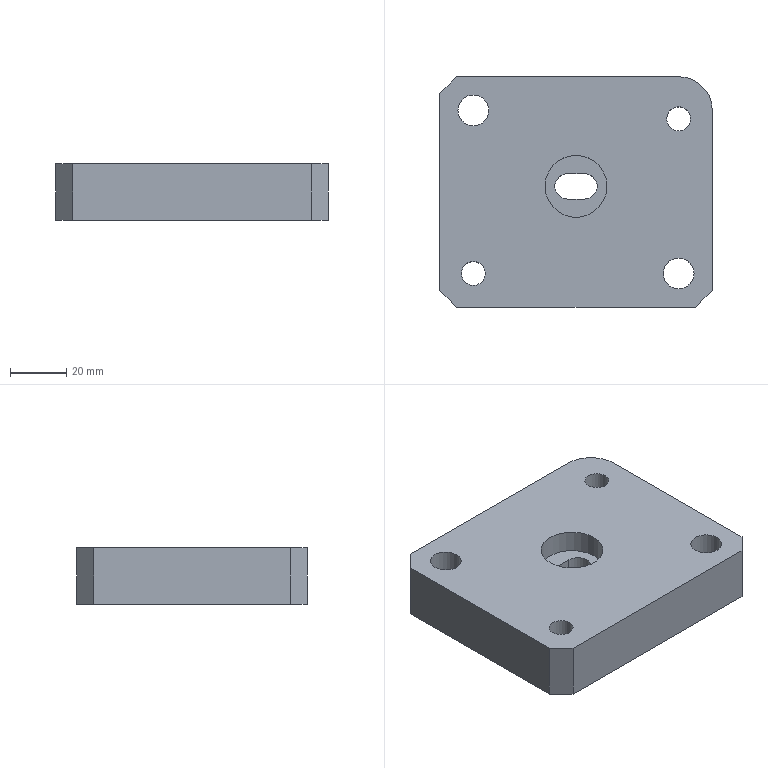Part | STEP file | lll_id3586_x_t | 1 solid | 28 faces | box 97 x 82 x 20 mm | volume 143143 mm3 | plane 16 | cylinder 12 | commonest cylinder face diameters 11 x4 8.5 x2 9.05 x2 17 x2 22 x1 24 x1
STEP:
#1=CARTESIAN_POINT('',(3545.234,257.45,22.5));
#2=VERTEX_POINT('',#1);
#3=CARTESIAN_POINT('',(3550.734,257.45,22.5));
#4=DIRECTION('',(0.,0.,-1.));
#5=DIRECTION('',(-1.,0.,0.));
#6=AXIS2_PLACEMENT_3D('',#3,#4,#5);
#7=CIRCLE('',#6,5.5);
#8=EDGE_CURVE('',#2,#2,#7,.T.);
#9=ORIENTED_EDGE('',*,*,#8,.T.);
#10=EDGE_LOOP('',(#9));
#11=FACE_BOUND('',#10,.T.);
#12=CARTESIAN_POINT('',(3635.734,193.45,22.5));
#13=VERTEX_POINT('',#12);
#14=CARTESIAN_POINT('',(3635.734,257.45,22.5));
#15=VERTEX_POINT('',#14);
#16=CARTESIAN_POINT('',(3635.734,221.45,22.5));
#17=DIRECTION('',(0.,1.,0.));
#18=VECTOR('',#17,1.);
#19=LINE('',#16,#18);
#20=EDGE_CURVE('',#13,#15,#19,.T.);
#21=ORIENTED_EDGE('',*,*,#20,.T.);
#22=CARTESIAN_POINT('',(3623.734,269.45,22.5));
#23=VERTEX_POINT('',#22);
#24=CARTESIAN_POINT('',(3623.734,257.45,22.5));
#25=DIRECTION('',(0.,0.,1.));
#26=DIRECTION('',(1.,0.,0.));
#27=AXIS2_PLACEMENT_3D('',#24,#25,#26);
#28=CIRCLE('',#27,12.);
#29=EDGE_CURVE('',#15,#23,#28,.T.);
#30=ORIENTED_EDGE('',*,*,#29,.T.);
#31=CARTESIAN_POINT('',(3544.734,269.45,22.5));
#32=VERTEX_POINT('',#31);
#33=CARTESIAN_POINT('',(3589.234,269.45,22.5));
#34=DIRECTION('',(-1.,0.,0.));
#35=VECTOR('',#34,1.);
#36=LINE('',#33,#35);
#37=EDGE_CURVE('',#23,#32,#36,.T.);
#38=ORIENTED_EDGE('',*,*,#37,.T.);
#39=CARTESIAN_POINT('',(3538.734,263.45,22.5));
#40=VERTEX_POINT('',#39);
#41=CARTESIAN_POINT('',(3683.114,407.83,22.5));
#42=DIRECTION('',(-0.7071,-0.7071,0.));
#43=VECTOR('',#42,1.);
#44=LINE('',#41,#43);
#45=EDGE_CURVE('',#32,#40,#44,.T.);
#46=ORIENTED_EDGE('',*,*,#45,.T.);
#47=CARTESIAN_POINT('',(3538.734,193.45,22.5));
#48=VERTEX_POINT('',#47);
#49=CARTESIAN_POINT('',(3538.734,192.292,22.5));
#50=DIRECTION('',(0.,1.,0.));
#51=VECTOR('',#50,1.);
#52=LINE('',#49,#51);
#53=EDGE_CURVE('',#48,#40,#52,.T.);
#54=ORIENTED_EDGE('',*,*,#53,.F.);
#55=CARTESIAN_POINT('',(3544.734,187.45,22.5));
#56=VERTEX_POINT('',#55);
#57=CARTESIAN_POINT('',(3719.271,12.913,22.5));
#58=DIRECTION('',(0.7071,-0.7071,0.));
#59=VECTOR('',#58,1.);
#60=LINE('',#57,#59);
#61=EDGE_CURVE('',#48,#56,#60,.T.);
#62=ORIENTED_EDGE('',*,*,#61,.T.);
#63=CARTESIAN_POINT('',(3629.734,187.45,22.5));
#64=VERTEX_POINT('',#63);
#65=CARTESIAN_POINT('',(3589.234,187.45,22.5));
#66=DIRECTION('',(1.,0.,0.));
#67=VECTOR('',#66,1.);
#68=LINE('',#65,#67);
#69=EDGE_CURVE('',#56,#64,#68,.T.);
#70=ORIENTED_EDGE('',*,*,#69,.T.);
#71=CARTESIAN_POINT('',(3766.614,324.33,22.5));
#72=DIRECTION('',(0.7071,0.7071,0.));
#73=VECTOR('',#72,1.);
#74=LINE('',#71,#73);
#75=EDGE_CURVE('',#64,#13,#74,.T.);
#76=ORIENTED_EDGE('',*,*,#75,.T.);
#77=EDGE_LOOP('',(#21,#30,#38,#46,#54,#62,#70,#76));
#78=FACE_BOUND('',#77,.T.);
#79=CARTESIAN_POINT('',(3618.234,199.45,22.5));
#80=VERTEX_POINT('',#79);
#81=CARTESIAN_POINT('',(3623.734,199.45,22.5));
#82=DIRECTION('',(0.,0.,-1.));
#83=DIRECTION('',(-1.,0.,0.));
#84=AXIS2_PLACEMENT_3D('',#81,#82,#83);
#85=CIRCLE('',#84,5.5);
#86=EDGE_CURVE('',#80,#80,#85,.T.);
#87=ORIENTED_EDGE('',*,*,#86,.T.);
#88=EDGE_LOOP('',(#87));
#89=FACE_BOUND('',#88,.T.);
#90=CARTESIAN_POINT('',(3546.484,199.45,22.5));
#91=VERTEX_POINT('',#90);
#92=CARTESIAN_POINT('',(3550.734,199.45,22.5));
#93=DIRECTION('',(0.,0.,-1.));
#94=DIRECTION('',(-1.,0.,0.));
#95=AXIS2_PLACEMENT_3D('',#92,#93,#94);
#96=CIRCLE('',#95,4.25);
#97=EDGE_CURVE('',#91,#91,#96,.T.);
#98=ORIENTED_EDGE('',*,*,#97,.T.);
#99=EDGE_LOOP('',(#98));
#100=FACE_BOUND('',#99,.T.);
#101=CARTESIAN_POINT('',(3619.484,254.45,22.5));
#102=VERTEX_POINT('',#101);
#103=CARTESIAN_POINT('',(3623.734,254.45,22.5));
#104=DIRECTION('',(0.,0.,-1.));
#105=DIRECTION('',(-1.,0.,0.));
#106=AXIS2_PLACEMENT_3D('',#103,#104,#105);
#107=CIRCLE('',#106,4.25);
#108=EDGE_CURVE('',#102,#102,#107,.T.);
#109=ORIENTED_EDGE('',*,*,#108,.T.);
#110=EDGE_LOOP('',(#109));
#111=FACE_BOUND('',#110,.T.);
#112=CARTESIAN_POINT('',(3576.234,230.45,22.5));
#113=VERTEX_POINT('',#112);
#114=CARTESIAN_POINT('',(3587.234,230.45,22.5));
#115=DIRECTION('',(0.,0.,-1.));
#116=DIRECTION('',(-1.,0.,0.));
#117=AXIS2_PLACEMENT_3D('',#114,#115,#116);
#118=CIRCLE('',#117,11.);
#119=EDGE_CURVE('',#113,#113,#118,.T.);
#120=ORIENTED_EDGE('',*,*,#119,.T.);
#121=EDGE_LOOP('',(#120));
#122=FACE_BOUND('',#121,.T.);
#123=CARTESIAN_POINT('',(3898.651,192.292,22.5));
#124=DIRECTION('',(0.,0.,1.));
#125=DIRECTION('',(0.,-1.,0.));
#126=AXIS2_PLACEMENT_3D('',#123,#124,#125);
#127=PLANE('',#126);
#128=ADVANCED_FACE('',(#11,#78,#89,#100,#111,#122),#127,.T.);
#129=CARTESIAN_POINT('',(3590.234,225.925,14.5));
#130=VERTEX_POINT('',#129);
#131=CARTESIAN_POINT('',(3590.234,225.925,2.5));
#132=VERTEX_POINT('',#131);
#133=CARTESIAN_POINT('',(3590.234,225.925,2.5));
#134=DIRECTION('',(0.000000008,0.,-1.));
#135=VECTOR('',#134,1.);
#136=LINE('',#133,#135);
#137=EDGE_CURVE('',#130,#132,#136,.T.);
#138=ORIENTED_EDGE('',*,*,#137,.F.);
#139=CARTESIAN_POINT('',(3590.234,234.975,14.5));
#140=VERTEX_POINT('',#139);
#141=CARTESIAN_POINT('',(3590.234,230.45,14.5));
#142=DIRECTION('',(0.,0.,1.));
#143=DIRECTION('',(1.,0.,0.));
#144=AXIS2_PLACEMENT_3D('',#141,#142,#143);
#145=CIRCLE('',#144,4.525);
#146=EDGE_CURVE('',#130,#140,#145,.T.);
#147=ORIENTED_EDGE('',*,*,#146,.T.);
#148=CARTESIAN_POINT('',(3590.234,234.975,2.5));
#149=VERTEX_POINT('',#148);
#150=CARTESIAN_POINT('',(3590.234,234.975,2.5));
#151=DIRECTION('',(0.000000008,0.,-1.));
#152=VECTOR('',#151,1.);
#153=LINE('',#150,#152);
#154=EDGE_CURVE('',#140,#149,#153,.T.);
#155=ORIENTED_EDGE('',*,*,#154,.T.);
#156=CARTESIAN_POINT('',(3590.234,230.45,2.5));
#157=DIRECTION('',(0.,0.,-1.));
#158=DIRECTION('',(-1.,0.,0.));
#159=AXIS2_PLACEMENT_3D('',#156,#157,#158);
#160=CIRCLE('',#159,4.525);
#161=EDGE_CURVE('',#149,#132,#160,.T.);
#162=ORIENTED_EDGE('',*,*,#161,.T.);
#163=EDGE_LOOP('',(#138,#147,#155,#162));
#164=FACE_OUTER_BOUND('',#163,.T.);
#165=CARTESIAN_POINT('',(3590.234,230.45,2.5));
#166=DIRECTION('',(-0.000000008,0.,1.));
#167=DIRECTION('',(-1.,0.,-0.000000008));
#168=AXIS2_PLACEMENT_3D('',#165,#166,#167);
#169=CYLINDRICAL_SURFACE('',#168,4.525);
#170=ADVANCED_FACE('',(#164),#169,.F.);
#171=ORIENTED_EDGE('',*,*,#154,.F.);
#172=CARTESIAN_POINT('',(3584.234,234.975,14.5));
#173=VERTEX_POINT('',#172);
#174=CARTESIAN_POINT('',(3584.234,234.975,14.5));
#175=DIRECTION('',(-1.,0.,0.));
#176=VECTOR('',#175,1.);
#177=LINE('',#174,#176);
#178=EDGE_CURVE('',#140,#173,#177,.T.);
#179=ORIENTED_EDGE('',*,*,#178,.T.);
#180=CARTESIAN_POINT('',(3584.234,234.975,2.5));
#181=VERTEX_POINT('',#180);
#182=CARTESIAN_POINT('',(3584.234,234.975,2.5));
#183=DIRECTION('',(0.000000008,0.,-1.));
#184=VECTOR('',#183,1.);
#185=LINE('',#182,#184);
#186=EDGE_CURVE('',#173,#181,#185,.T.);
#187=ORIENTED_EDGE('',*,*,#186,.T.);
#188=CARTESIAN_POINT('',(3898.651,234.975,2.5));
#189=DIRECTION('',(1.,0.,0.));
#190=VECTOR('',#189,1.);
#191=LINE('',#188,#190);
#192=EDGE_CURVE('',#181,#149,#191,.T.);
#193=ORIENTED_EDGE('',*,*,#192,.T.);
#194=EDGE_LOOP('',(#171,#179,#187,#193));
#195=FACE_OUTER_BOUND('',#194,.T.);
#196=CARTESIAN_POINT('',(3584.234,234.975,2.5));
#197=DIRECTION('',(0.,-1.,0.));
#198=DIRECTION('',(1.,0.,0.000000008));
#199=AXIS2_PLACEMENT_3D('',#196,#197,#198);
#200=PLANE('',#199);
#201=ADVANCED_FACE('',(#195),#200,.T.);
#202=ORIENTED_EDGE('',*,*,#186,.F.);
#203=CARTESIAN_POINT('',(3584.234,225.925,14.5));
#204=VERTEX_POINT('',#203);
#205=CARTESIAN_POINT('',(3584.234,230.45,14.5));
#206=DIRECTION('',(0.,0.,1.));
#207=DIRECTION('',(1.,0.,0.));
#208=AXIS2_PLACEMENT_3D('',#205,#206,#207);
#209=CIRCLE('',#208,4.525);
#210=EDGE_CURVE('',#173,#204,#209,.T.);
#211=ORIENTED_EDGE('',*,*,#210,.T.);
#212=CARTESIAN_POINT('',(3584.234,225.925,2.5));
#213=VERTEX_POINT('',#212);
#214=CARTESIAN_POINT('',(3584.234,225.925,2.5));
#215=DIRECTION('',(0.000000008,0.,-1.));
#216=VECTOR('',#215,1.);
#217=LINE('',#214,#216);
#218=EDGE_CURVE('',#204,#213,#217,.T.);
#219=ORIENTED_EDGE('',*,*,#218,.T.);
#220=CARTESIAN_POINT('',(3584.234,230.45,2.5));
#221=DIRECTION('',(0.,0.,-1.));
#222=DIRECTION('',(-1.,0.,0.));
#223=AXIS2_PLACEMENT_3D('',#220,#221,#222);
#224=CIRCLE('',#223,4.525);
#225=EDGE_CURVE('',#213,#181,#224,.T.);
#226=ORIENTED_EDGE('',*,*,#225,.T.);
#227=EDGE_LOOP('',(#202,#211,#219,#226));
#228=FACE_OUTER_BOUND('',#227,.T.);
#229=CARTESIAN_POINT('',(3584.234,230.45,2.5));
#230=DIRECTION('',(-0.000000008,0.,1.));
#231=DIRECTION('',(-1.,0.,-0.000000008));
#232=AXIS2_PLACEMENT_3D('',#229,#230,#231);
#233=CYLINDRICAL_SURFACE('',#232,4.525);
#234=ADVANCED_FACE('',(#228),#233,.F.);
#235=ORIENTED_EDGE('',*,*,#218,.F.);
#236=CARTESIAN_POINT('',(3584.234,225.925,14.5));
#237=DIRECTION('',(1.,0.,0.));
#238=VECTOR('',#237,1.);
#239=LINE('',#236,#238);
#240=EDGE_CURVE('',#204,#130,#239,.T.);
#241=ORIENTED_EDGE('',*,*,#240,.T.);
#242=ORIENTED_EDGE('',*,*,#137,.T.);
#243=CARTESIAN_POINT('',(3898.651,225.925,2.5));
#244=DIRECTION('',(-1.,0.,0.));
#245=VECTOR('',#244,1.);
#246=LINE('',#243,#245);
#247=EDGE_CURVE('',#132,#213,#246,.T.);
#248=ORIENTED_EDGE('',*,*,#247,.T.);
#249=EDGE_LOOP('',(#235,#241,#242,#248));
#250=FACE_OUTER_BOUND('',#249,.T.);
#251=CARTESIAN_POINT('',(3584.234,225.925,2.5));
#252=DIRECTION('',(0.,-1.,0.));
#253=DIRECTION('',(1.,0.,0.000000008));
#254=AXIS2_PLACEMENT_3D('',#251,#252,#253);
#255=PLANE('',#254);
#256=ADVANCED_FACE('',(#250),#255,.F.);
#257=ORIENTED_EDGE('',*,*,#161,.F.);
#258=ORIENTED_EDGE('',*,*,#192,.F.);
#259=ORIENTED_EDGE('',*,*,#225,.F.);
#260=ORIENTED_EDGE('',*,*,#247,.F.);
#261=EDGE_LOOP('',(#257,#258,#259,#260));
#262=FACE_BOUND('',#261,.T.);
#263=CARTESIAN_POINT('',(3545.234,199.45,2.5));
#264=VERTEX_POINT('',#263);
#265=CARTESIAN_POINT('',(3550.734,199.45,2.5));
#266=DIRECTION('',(0.,0.,-1.));
#267=DIRECTION('',(-1.,0.,0.));
#268=AXIS2_PLACEMENT_3D('',#265,#266,#267);
#269=CIRCLE('',#268,5.5);
#270=EDGE_CURVE('',#264,#264,#269,.T.);
#271=ORIENTED_EDGE('',*,*,#270,.F.);
#272=EDGE_LOOP('',(#271));
#273=FACE_BOUND('',#272,.T.);
#274=CARTESIAN_POINT('',(3615.234,199.45,2.5));
#275=VERTEX_POINT('',#274);
#276=CARTESIAN_POINT('',(3623.734,199.45,2.5));
#277=DIRECTION('',(0.,0.,1.));
#278=DIRECTION('',(-1.,0.,0.));
#279=AXIS2_PLACEMENT_3D('',#276,#277,#278);
#280=CIRCLE('',#279,8.5);
#281=EDGE_CURVE('',#275,#275,#280,.T.);
#282=ORIENTED_EDGE('',*,*,#281,.T.);
#283=EDGE_LOOP('',(#282));
#284=FACE_BOUND('',#283,.T.);
#285=CARTESIAN_POINT('',(3544.734,269.45,2.5));
#286=VERTEX_POINT('',#285);
#287=CARTESIAN_POINT('',(3623.734,269.45,2.5));
#288=VERTEX_POINT('',#287);
#289=CARTESIAN_POINT('',(3589.234,269.45,2.5));
#290=DIRECTION('',(1.,0.,0.));
#291=VECTOR('',#290,1.);
#292=LINE('',#289,#291);
#293=EDGE_CURVE('',#286,#288,#292,.T.);
#294=ORIENTED_EDGE('',*,*,#293,.T.);
#295=CARTESIAN_POINT('',(3635.734,257.45,2.5));
#296=VERTEX_POINT('',#295);
#297=CARTESIAN_POINT('',(3623.734,257.45,2.5));
#298=DIRECTION('',(0.,0.,-1.));
#299=DIRECTION('',(1.,0.,0.));
#300=AXIS2_PLACEMENT_3D('',#297,#298,#299);
#301=CIRCLE('',#300,12.);
#302=EDGE_CURVE('',#288,#296,#301,.T.);
#303=ORIENTED_EDGE('',*,*,#302,.T.);
#304=CARTESIAN_POINT('',(3635.734,193.45,2.5));
#305=VERTEX_POINT('',#304);
#306=CARTESIAN_POINT('',(3635.734,221.45,2.5));
#307=DIRECTION('',(0.,-1.,0.));
#308=VECTOR('',#307,1.);
#309=LINE('',#306,#308);
#310=EDGE_CURVE('',#296,#305,#309,.T.);
#311=ORIENTED_EDGE('',*,*,#310,.T.);
#312=CARTESIAN_POINT('',(3629.734,187.45,2.5));
#313=VERTEX_POINT('',#312);
#314=CARTESIAN_POINT('',(3635.734,193.45,2.5));
#315=DIRECTION('',(-0.7071,-0.7071,0.));
#316=VECTOR('',#315,1.);
#317=LINE('',#314,#316);
#318=EDGE_CURVE('',#305,#313,#317,.T.);
#319=ORIENTED_EDGE('',*,*,#318,.T.);
#320=CARTESIAN_POINT('',(3544.734,187.45,2.5));
#321=VERTEX_POINT('',#320);
#322=CARTESIAN_POINT('',(3589.234,187.45,2.5));
#323=DIRECTION('',(-1.,0.,0.));
#324=VECTOR('',#323,1.);
#325=LINE('',#322,#324);
#326=EDGE_CURVE('',#313,#321,#325,.T.);
#327=ORIENTED_EDGE('',*,*,#326,.T.);
#328=CARTESIAN_POINT('',(3538.734,193.45,2.5));
#329=VERTEX_POINT('',#328);
#330=CARTESIAN_POINT('',(3544.734,187.45,2.5));
#331=DIRECTION('',(-0.7071,0.7071,0.));
#332=VECTOR('',#331,1.);
#333=LINE('',#330,#332);
#334=EDGE_CURVE('',#321,#329,#333,.T.);
#335=ORIENTED_EDGE('',*,*,#334,.T.);
#336=CARTESIAN_POINT('',(3538.734,263.45,2.5));
#337=VERTEX_POINT('',#336);
#338=CARTESIAN_POINT('',(3538.734,192.292,2.5));
#339=DIRECTION('',(0.,-1.,0.));
#340=VECTOR('',#339,1.);
#341=LINE('',#338,#340);
#342=EDGE_CURVE('',#337,#329,#341,.T.);
#343=ORIENTED_EDGE('',*,*,#342,.F.);
#344=CARTESIAN_POINT('',(3544.734,269.45,2.5));
#345=DIRECTION('',(0.7071,0.7071,0.));
#346=VECTOR('',#345,1.);
#347=LINE('',#344,#346);
#348=EDGE_CURVE('',#337,#286,#347,.T.);
#349=ORIENTED_EDGE('',*,*,#348,.T.);
#350=EDGE_LOOP('',(#294,#303,#311,#319,#327,#335,#343,#349));
#351=FACE_BOUND('',#350,.T.);
#352=CARTESIAN_POINT('',(3542.234,257.45,2.5));
#353=VERTEX_POINT('',#352);
#354=CARTESIAN_POINT('',(3550.734,257.45,2.5));
#355=DIRECTION('',(0.,0.,-1.));
#356=DIRECTION('',(-1.,0.,0.));
#357=AXIS2_PLACEMENT_3D('',#354,#355,#356);
#358=CIRCLE('',#357,8.5);
#359=EDGE_CURVE('',#353,#353,#358,.T.);
#360=ORIENTED_EDGE('',*,*,#359,.F.);
#361=EDGE_LOOP('',(#360));
#362=FACE_BOUND('',#361,.T.);
#363=CARTESIAN_POINT('',(3618.234,254.45,2.5));
#364=VERTEX_POINT('',#363);
#365=CARTESIAN_POINT('',(3623.734,254.45,2.5));
#366=DIRECTION('',(0.,0.,1.));
#367=DIRECTION('',(-1.,0.,0.));
#368=AXIS2_PLACEMENT_3D('',#365,#366,#367);
#369=CIRCLE('',#368,5.5);
#370=EDGE_CURVE('',#364,#364,#369,.T.);
#371=ORIENTED_EDGE('',*,*,#370,.T.);
#372=EDGE_LOOP('',(#371));
#373=FACE_BOUND('',#372,.T.);
#374=CARTESIAN_POINT('',(3898.651,192.292,2.5));
#375=DIRECTION('',(0.,0.,1.));
#376=DIRECTION('',(0.,-1.,0.));
#377=AXIS2_PLACEMENT_3D('',#374,#375,#376);
#378=PLANE('',#377);
#379=ADVANCED_FACE('',(#262,#273,#284,#351,#362,#373),#378,.F.);
#380=CARTESIAN_POINT('',(3546.484,199.45,9.5));
#381=VERTEX_POINT('',#380);
#382=CARTESIAN_POINT('',(3550.734,199.45,9.5));
#383=DIRECTION('',(0.,0.,1.));
#384=DIRECTION('',(-1.,0.,0.));
#385=AXIS2_PLACEMENT_3D('',#382,#383,#384);
#386=CIRCLE('',#385,4.25);
#387=EDGE_CURVE('',#381,#381,#386,.T.);
#388=ORIENTED_EDGE('',*,*,#387,.T.);
#389=EDGE_LOOP('',(#388));
#390=FACE_BOUND('',#389,.T.);
#391=CARTESIAN_POINT('',(3545.234,199.45,9.5));
#392=VERTEX_POINT('',#391);
#393=CARTESIAN_POINT('',(3550.734,199.45,9.5));
#394=DIRECTION('',(0.,0.,1.));
#395=DIRECTION('',(-1.,0.,0.));
#396=AXIS2_PLACEMENT_3D('',#393,#394,#395);
#397=CIRCLE('',#396,5.5);
#398=EDGE_CURVE('',#392,#392,#397,.T.);
#399=ORIENTED_EDGE('',*,*,#398,.F.);
#400=EDGE_LOOP('',(#399));
#401=FACE_BOUND('',#400,.T.);
#402=CARTESIAN_POINT('',(3550.734,199.45,9.5));
#403=DIRECTION('',(0.,0.,1.));
#404=DIRECTION('',(-1.,0.,0.));
#405=AXIS2_PLACEMENT_3D('',#402,#403,#404);
#406=PLANE('',#405);
#407=ADVANCED_FACE('',(#390,#401),#406,.F.);
#408=CARTESIAN_POINT('',(3618.234,199.45,14.5));
#409=VERTEX_POINT('',#408);
#410=CARTESIAN_POINT('',(3623.734,199.45,14.5));
#411=DIRECTION('',(0.,0.,-1.));
#412=DIRECTION('',(-1.,0.,0.));
#413=AXIS2_PLACEMENT_3D('',#410,#411,#412);
#414=CIRCLE('',#413,5.5);
#415=EDGE_CURVE('',#409,#409,#414,.T.);
#416=ORIENTED_EDGE('',*,*,#415,.F.);
#417=EDGE_LOOP('',(#416));
#418=FACE_BOUND('',#417,.T.);
#419=CARTESIAN_POINT('',(3615.234,199.45,14.5));
#420=VERTEX_POINT('',#419);
#421=CARTESIAN_POINT('',(3623.734,199.45,14.5));
#422=DIRECTION('',(0.,0.,-1.));
#423=DIRECTION('',(-1.,0.,0.));
#424=AXIS2_PLACEMENT_3D('',#421,#422,#423);
#425=CIRCLE('',#424,8.5);
#426=EDGE_CURVE('',#420,#420,#425,.T.);
#427=ORIENTED_EDGE('',*,*,#426,.T.);
#428=EDGE_LOOP('',(#427));
#429=FACE_BOUND('',#428,.T.);
#430=CARTESIAN_POINT('',(3623.734,199.45,14.5));
#431=DIRECTION('',(0.,0.,1.));
#432=DIRECTION('',(0.,1.,0.));
#433=AXIS2_PLACEMENT_3D('',#430,#431,#432);
#434=PLANE('',#433);
#435=ADVANCED_FACE('',(#418,#429),#434,.F.);
#436=CARTESIAN_POINT('',(3545.234,257.45,14.5));
#437=VERTEX_POINT('',#436);
#438=CARTESIAN_POINT('',(3550.734,257.45,14.5));
#439=DIRECTION('',(0.,0.,1.));
#440=DIRECTION('',(-1.,0.,0.));
#441=AXIS2_PLACEMENT_3D('',#438,#439,#440);
#442=CIRCLE('',#441,5.5);
#443=EDGE_CURVE('',#437,#437,#442,.T.);
#444=ORIENTED_EDGE('',*,*,#443,.T.);
#445=EDGE_LOOP('',(#444));
#446=FACE_BOUND('',#445,.T.);
#447=CARTESIAN_POINT('',(3542.234,257.45,14.5));
#448=VERTEX_POINT('',#447);
#449=CARTESIAN_POINT('',(3550.734,257.45,14.5));
#450=DIRECTION('',(0.,0.,1.));
#451=DIRECTION('',(-1.,0.,0.));
#452=AXIS2_PLACEMENT_3D('',#449,#450,#451);
#453=CIRCLE('',#452,8.5);
#454=EDGE_CURVE('',#448,#448,#453,.T.);
#455=ORIENTED_EDGE('',*,*,#454,.F.);
#456=EDGE_LOOP('',(#455));
#457=FACE_BOUND('',#456,.T.);
#458=CARTESIAN_POINT('',(3550.734,257.45,14.5));
#459=DIRECTION('',(0.,0.,1.));
#460=DIRECTION('',(0.,-1.,0.));
#461=AXIS2_PLACEMENT_3D('',#458,#459,#460);
#462=PLANE('',#461);
#463=ADVANCED_FACE('',(#446,#457),#462,.F.);
#464=ORIENTED_EDGE('',*,*,#8,.F.);
#465=EDGE_LOOP('',(#464));
#466=FACE_BOUND('',#465,.T.);
#467=ORIENTED_EDGE('',*,*,#443,.F.);
#468=EDGE_LOOP('',(#467));
#469=FACE_BOUND('',#468,.T.);
#470=CARTESIAN_POINT('',(3550.734,257.45,97.5));
#471=DIRECTION('',(0.,0.,1.));
#472=DIRECTION('',(0.,-1.,0.));
#473=AXIS2_PLACEMENT_3D('',#470,#471,#472);
#474=CYLINDRICAL_SURFACE('',#473,5.5);
#475=ADVANCED_FACE('',(#466,#469),#474,.F.);
#476=ORIENTED_EDGE('',*,*,#398,.T.);
#477=EDGE_LOOP('',(#476));
#478=FACE_BOUND('',#477,.T.);
#479=ORIENTED_EDGE('',*,*,#270,.T.);
#480=EDGE_LOOP('',(#479));
#481=FACE_BOUND('',#480,.T.);
#482=CARTESIAN_POINT('',(3550.734,199.45,-2.5));
#483=DIRECTION('',(0.,0.,1.));
#484=DIRECTION('',(-1.,0.,0.));
#485=AXIS2_PLACEMENT_3D('',#482,#483,#484);
#486=CYLINDRICAL_SURFACE('',#485,5.5);
#487=ADVANCED_FACE('',(#478,#481),#486,.F.);
#488=ORIENTED_EDGE('',*,*,#426,.F.);
#489=EDGE_LOOP('',(#488));
#490=FACE_BOUND('',#489,.T.);
#491=ORIENTED_EDGE('',*,*,#281,.F.);
#492=EDGE_LOOP('',(#491));
#493=FACE_BOUND('',#492,.T.);
#494=CARTESIAN_POINT('',(3623.734,199.45,-2.5));
#495=DIRECTION('',(0.,0.,1.));
#496=DIRECTION('',(0.,1.,0.));
#497=AXIS2_PLACEMENT_3D('',#494,#495,#496);
#498=CYLINDRICAL_SURFACE('',#497,8.5);
#499=ADVANCED_FACE('',(#490,#493),#498,.F.);
#500=ORIENTED_EDGE('',*,*,#310,.F.);
#501=CARTESIAN_POINT('',(3635.734,257.45,-81.5));
#502=DIRECTION('',(0.,0.,1.));
#503=VECTOR('',#502,1.);
#504=LINE('',#501,#503);
#505=EDGE_CURVE('',#296,#15,#504,.T.);
#506=ORIENTED_EDGE('',*,*,#505,.T.);
#507=ORIENTED_EDGE('',*,*,#20,.F.);
#508=CARTESIAN_POINT('',(3635.734,193.45,-81.5));
#509=DIRECTION('',(0.,0.,-1.));
#510=VECTOR('',#509,1.);
#511=LINE('',#508,#510);
#512=EDGE_CURVE('',#13,#305,#511,.T.);
#513=ORIENTED_EDGE('',*,*,#512,.T.);
#514=EDGE_LOOP('',(#500,#506,#507,#513));
#515=FACE_OUTER_BOUND('',#514,.T.);
#516=CARTESIAN_POINT('',(3635.734,221.45,-81.5));
#517=DIRECTION('',(1.,0.,0.));
#518=DIRECTION('',(0.,0.,-1.));
#519=AXIS2_PLACEMENT_3D('',#516,#517,#518);
#520=PLANE('',#519);
#521=ADVANCED_FACE('',(#515),#520,.T.);
#522=ORIENTED_EDGE('',*,*,#326,.F.);
#523=CARTESIAN_POINT('',(3629.734,187.45,-81.5));
#524=DIRECTION('',(0.,0.,1.));
#525=VECTOR('',#524,1.);
#526=LINE('',#523,#525);
#527=EDGE_CURVE('',#313,#64,#526,.T.);
#528=ORIENTED_EDGE('',*,*,#527,.T.);
#529=ORIENTED_EDGE('',*,*,#69,.F.);
#530=CARTESIAN_POINT('',(3544.734,187.45,-81.5));
#531=DIRECTION('',(0.,0.,-1.));
#532=VECTOR('',#531,1.);
#533=LINE('',#530,#532);
#534=EDGE_CURVE('',#56,#321,#533,.T.);
#535=ORIENTED_EDGE('',*,*,#534,.T.);
#536=EDGE_LOOP('',(#522,#528,#529,#535));
#537=FACE_OUTER_BOUND('',#536,.T.);
#538=CARTESIAN_POINT('',(3589.234,187.45,-81.5));
#539=DIRECTION('',(0.,-1.,0.));
#540=DIRECTION('',(0.,0.,-1.));
#541=AXIS2_PLACEMENT_3D('',#538,#539,#540);
#542=PLANE('',#541);
#543=ADVANCED_FACE('',(#537),#542,.T.);
#544=ORIENTED_EDGE('',*,*,#53,.T.);
#545=CARTESIAN_POINT('',(3538.734,263.45,13.5));
#546=DIRECTION('',(0.,0.,-1.));
#547=VECTOR('',#546,1.);
#548=LINE('',#545,#547);
#549=EDGE_CURVE('',#40,#337,#548,.T.);
#550=ORIENTED_EDGE('',*,*,#549,.T.);
#551=ORIENTED_EDGE('',*,*,#342,.T.);
#552=CARTESIAN_POINT('',(3538.734,193.45,13.5));
#553=DIRECTION('',(0.,0.,1.));
#554=VECTOR('',#553,1.);
#555=LINE('',#552,#554);
#556=EDGE_CURVE('',#329,#48,#555,.T.);
#557=ORIENTED_EDGE('',*,*,#556,.T.);
#558=EDGE_LOOP('',(#544,#550,#551,#557));
#559=FACE_OUTER_BOUND('',#558,.T.);
#560=CARTESIAN_POINT('',(3538.734,221.45,13.5));
#561=DIRECTION('',(-1.,0.,0.));
#562=DIRECTION('',(0.,0.,1.));
#563=AXIS2_PLACEMENT_3D('',#560,#561,#562);
#564=PLANE('',#563);
#565=ADVANCED_FACE('',(#559),#564,.T.);
#566=ORIENTED_EDGE('',*,*,#37,.F.);
#567=CARTESIAN_POINT('',(3623.734,269.45,-81.5));
#568=DIRECTION('',(0.,0.,-1.));
#569=VECTOR('',#568,1.);
#570=LINE('',#567,#569);
#571=EDGE_CURVE('',#23,#288,#570,.T.);
#572=ORIENTED_EDGE('',*,*,#571,.T.);
#573=ORIENTED_EDGE('',*,*,#293,.F.);
#574=CARTESIAN_POINT('',(3544.734,269.45,-81.5));
#575=DIRECTION('',(0.,0.,1.));
#576=VECTOR('',#575,1.);
#577=LINE('',#574,#576);
#578=EDGE_CURVE('',#286,#32,#577,.T.);
#579=ORIENTED_EDGE('',*,*,#578,.T.);
#580=EDGE_LOOP('',(#566,#572,#573,#579));
#581=FACE_OUTER_BOUND('',#580,.T.);
#582=CARTESIAN_POINT('',(3589.234,269.45,-81.5));
#583=DIRECTION('',(0.,1.,0.));
#584=DIRECTION('',(0.,0.,1.));
#585=AXIS2_PLACEMENT_3D('',#582,#583,#584);
#586=PLANE('',#585);
#587=ADVANCED_FACE('',(#581),#586,.T.);
#588=ORIENTED_EDGE('',*,*,#454,.T.);
#589=EDGE_LOOP('',(#588));
#590=FACE_BOUND('',#589,.T.);
#591=ORIENTED_EDGE('',*,*,#359,.T.);
#592=EDGE_LOOP('',(#591));
#593=FACE_BOUND('',#592,.T.);
#594=CARTESIAN_POINT('',(3550.734,257.45,-2.5));
#595=DIRECTION('',(0.,0.,1.));
#596=DIRECTION('',(0.,-1.,0.));
#597=AXIS2_PLACEMENT_3D('',#594,#595,#596);
#598=CYLINDRICAL_SURFACE('',#597,8.5);
#599=ADVANCED_FACE('',(#590,#593),#598,.F.);
#600=ORIENTED_EDGE('',*,*,#86,.F.);
#601=EDGE_LOOP('',(#600));
#602=FACE_BOUND('',#601,.T.);
#603=ORIENTED_EDGE('',*,*,#415,.T.);
#604=EDGE_LOOP('',(#603));
#605=FACE_BOUND('',#604,.T.);
#606=CARTESIAN_POINT('',(3623.734,199.45,97.5));
#607=DIRECTION('',(0.,0.,1.));
#608=DIRECTION('',(0.,1.,0.));
#609=AXIS2_PLACEMENT_3D('',#606,#607,#608);
#610=CYLINDRICAL_SURFACE('',#609,5.5);
#611=ADVANCED_FACE('',(#602,#605),#610,.F.);
#612=ORIENTED_EDGE('',*,*,#97,.F.);
#613=EDGE_LOOP('',(#612));
#614=FACE_BOUND('',#613,.T.);
#615=ORIENTED_EDGE('',*,*,#387,.F.);
#616=EDGE_LOOP('',(#615));
#617=FACE_BOUND('',#616,.T.);
#618=CARTESIAN_POINT('',(3550.734,199.45,97.5));
#619=DIRECTION('',(0.,0.,1.));
#620=DIRECTION('',(-1.,0.,0.));
#621=AXIS2_PLACEMENT_3D('',#618,#619,#620);
#622=CYLINDRICAL_SURFACE('',#621,4.25);
#623=ADVANCED_FACE('',(#614,#617),#622,.F.);
#624=ORIENTED_EDGE('',*,*,#108,.F.);
#625=EDGE_LOOP('',(#624));
#626=FACE_BOUND('',#625,.T.);
#627=CARTESIAN_POINT('',(3619.484,254.45,9.5));
#628=VERTEX_POINT('',#627);
#629=CARTESIAN_POINT('',(3623.734,254.45,9.5));
#630=DIRECTION('',(0.,0.,1.));
#631=DIRECTION('',(-1.,0.,0.));
#632=AXIS2_PLACEMENT_3D('',#629,#630,#631);
#633=CIRCLE('',#632,4.25);
#634=EDGE_CURVE('',#628,#628,#633,.T.);
#635=ORIENTED_EDGE('',*,*,#634,.F.);
#636=EDGE_LOOP('',(#635));
#637=FACE_BOUND('',#636,.T.);
#638=CARTESIAN_POINT('',(3623.734,254.45,97.5));
#639=DIRECTION('',(0.,0.,1.));
#640=DIRECTION('',(1.,0.,0.));
#641=AXIS2_PLACEMENT_3D('',#638,#639,#640);
#642=CYLINDRICAL_SURFACE('',#641,4.25);
#643=ADVANCED_FACE('',(#626,#637),#642,.F.);
#644=ORIENTED_EDGE('',*,*,#634,.T.);
#645=EDGE_LOOP('',(#644));
#646=FACE_BOUND('',#645,.T.);
#647=CARTESIAN_POINT('',(3618.234,254.45,9.5));
#648=VERTEX_POINT('',#647);
#649=CARTESIAN_POINT('',(3623.734,254.45,9.5));
#650=DIRECTION('',(0.,0.,1.));
#651=DIRECTION('',(-1.,0.,0.));
#652=AXIS2_PLACEMENT_3D('',#649,#650,#651);
#653=CIRCLE('',#652,5.5);
#654=EDGE_CURVE('',#648,#648,#653,.T.);
#655=ORIENTED_EDGE('',*,*,#654,.F.);
#656=EDGE_LOOP('',(#655));
#657=FACE_BOUND('',#656,.T.);
#658=CARTESIAN_POINT('',(3623.734,254.45,9.5));
#659=DIRECTION('',(0.,0.,1.));
#660=DIRECTION('',(1.,0.,0.));
#661=AXIS2_PLACEMENT_3D('',#658,#659,#660);
#662=PLANE('',#661);
#663=ADVANCED_FACE('',(#646,#657),#662,.F.);
#664=ORIENTED_EDGE('',*,*,#654,.T.);
#665=EDGE_LOOP('',(#664));
#666=FACE_BOUND('',#665,.T.);
#667=ORIENTED_EDGE('',*,*,#370,.F.);
#668=EDGE_LOOP('',(#667));
#669=FACE_BOUND('',#668,.T.);
#670=CARTESIAN_POINT('',(3623.734,254.45,-2.5));
#671=DIRECTION('',(0.,0.,1.));
#672=DIRECTION('',(1.,0.,0.));
#673=AXIS2_PLACEMENT_3D('',#670,#671,#672);
#674=CYLINDRICAL_SURFACE('',#673,5.5);
#675=ADVANCED_FACE('',(#666,#669),#674,.F.);
#676=CARTESIAN_POINT('',(3598.234,230.45,14.5));
#677=VERTEX_POINT('',#676);
#678=CARTESIAN_POINT('',(3587.234,230.45,14.5));
#679=DIRECTION('',(0.,0.,1.));
#680=DIRECTION('',(1.,0.,0.));
#681=AXIS2_PLACEMENT_3D('',#678,#679,#680);
#682=CIRCLE('',#681,11.);
#683=EDGE_CURVE('',#677,#677,#682,.T.);
#684=ORIENTED_EDGE('',*,*,#683,.T.);
#685=EDGE_LOOP('',(#684));
#686=FACE_BOUND('',#685,.T.);
#687=ORIENTED_EDGE('',*,*,#240,.F.);
#688=ORIENTED_EDGE('',*,*,#210,.F.);
#689=ORIENTED_EDGE('',*,*,#178,.F.);
#690=ORIENTED_EDGE('',*,*,#146,.F.);
#691=EDGE_LOOP('',(#687,#688,#689,#690));
#692=FACE_BOUND('',#691,.T.);
#693=CARTESIAN_POINT('',(3587.234,230.45,14.5));
#694=DIRECTION('',(0.,0.,-1.));
#695=DIRECTION('',(1.,0.,0.));
#696=AXIS2_PLACEMENT_3D('',#693,#694,#695);
#697=PLANE('',#696);
#698=ADVANCED_FACE('',(#686,#692),#697,.F.);
#699=ORIENTED_EDGE('',*,*,#119,.F.);
#700=EDGE_LOOP('',(#699));
#701=FACE_BOUND('',#700,.T.);
#702=ORIENTED_EDGE('',*,*,#683,.F.);
#703=EDGE_LOOP('',(#702));
#704=FACE_BOUND('',#703,.T.);
#705=CARTESIAN_POINT('',(3587.234,230.45,14.5));
#706=DIRECTION('',(0.,0.,1.));
#707=DIRECTION('',(-1.,0.,0.));
#708=AXIS2_PLACEMENT_3D('',#705,#706,#707);
#709=CYLINDRICAL_SURFACE('',#708,11.);
#710=ADVANCED_FACE('',(#701,#704),#709,.F.);
#711=ORIENTED_EDGE('',*,*,#348,.F.);
#712=ORIENTED_EDGE('',*,*,#549,.F.);
#713=ORIENTED_EDGE('',*,*,#45,.F.);
#714=ORIENTED_EDGE('',*,*,#578,.F.);
#715=EDGE_LOOP('',(#711,#712,#713,#714));
#716=FACE_OUTER_BOUND('',#715,.T.);
#717=CARTESIAN_POINT('',(3544.734,269.45,-81.5));
#718=DIRECTION('',(0.7071,-0.7071,0.));
#719=DIRECTION('',(0.,0.,-1.));
#720=AXIS2_PLACEMENT_3D('',#717,#718,#719);
#721=PLANE('',#720);
#722=ADVANCED_FACE('',(#716),#721,.F.);
#723=ORIENTED_EDGE('',*,*,#75,.F.);
#724=ORIENTED_EDGE('',*,*,#527,.F.);
#725=ORIENTED_EDGE('',*,*,#318,.F.);
#726=ORIENTED_EDGE('',*,*,#512,.F.);
#727=EDGE_LOOP('',(#723,#724,#725,#726));
#728=FACE_OUTER_BOUND('',#727,.T.);
#729=CARTESIAN_POINT('',(3635.734,193.45,-81.5));
#730=DIRECTION('',(-0.7071,0.7071,0.));
#731=DIRECTION('',(0.,0.,1.));
#732=AXIS2_PLACEMENT_3D('',#729,#730,#731);
#733=PLANE('',#732);
#734=ADVANCED_FACE('',(#728),#733,.F.);
#735=ORIENTED_EDGE('',*,*,#61,.F.);
#736=ORIENTED_EDGE('',*,*,#556,.F.);
#737=ORIENTED_EDGE('',*,*,#334,.F.);
#738=ORIENTED_EDGE('',*,*,#534,.F.);
#739=EDGE_LOOP('',(#735,#736,#737,#738));
#740=FACE_OUTER_BOUND('',#739,.T.);
#741=CARTESIAN_POINT('',(3544.734,187.45,-81.5));
#742=DIRECTION('',(0.7071,0.7071,0.));
#743=DIRECTION('',(0.,0.,1.));
#744=AXIS2_PLACEMENT_3D('',#741,#742,#743);
#745=PLANE('',#744);
#746=ADVANCED_FACE('',(#740),#745,.F.);
#747=ORIENTED_EDGE('',*,*,#29,.F.);
#748=ORIENTED_EDGE('',*,*,#505,.F.);
#749=ORIENTED_EDGE('',*,*,#302,.F.);
#750=ORIENTED_EDGE('',*,*,#571,.F.);
#751=EDGE_LOOP('',(#747,#748,#749,#750));
#752=FACE_OUTER_BOUND('',#751,.T.);
#753=CARTESIAN_POINT('',(3623.734,257.45,-81.5));
#754=DIRECTION('',(0.,0.,-1.));
#755=DIRECTION('',(1.,0.,0.));
#756=AXIS2_PLACEMENT_3D('',#753,#754,#755);
#757=CYLINDRICAL_SURFACE('',#756,12.);
#758=ADVANCED_FACE('',(#752),#757,.T.);
#759=CLOSED_SHELL('',(#128,#170,#201,#234,#256,#379,#407,#435,#463,#475,#487,#499,#521,#543,#565,#587,#599,#611,#623,#643,#663,#675,#698,#710,#722,#734,#746,#758));
#760=MANIFOLD_SOLID_BREP('',#759);
#761=(LENGTH_UNIT()NAMED_UNIT(*)SI_UNIT(.MILLI.,.METRE.));
#762=UNCERTAINTY_MEASURE_WITH_UNIT(LENGTH_MEASURE(0.00002),#761,'','');
#763=(NAMED_UNIT(*)PLANE_ANGLE_UNIT()SI_UNIT($,.RADIAN.));
#764=PLANE_ANGLE_MEASURE_WITH_UNIT(PLANE_ANGLE_MEASURE(0.01745),#763);
#765=DIMENSIONAL_EXPONENTS(0.,0.,0.,0.,0.,0.,0.);
#766=(CONVERSION_BASED_UNIT('DEGREE',#764)NAMED_UNIT(#765)PLANE_ANGLE_UNIT());
#767=(NAMED_UNIT(*)SI_UNIT($,.STERADIAN.)SOLID_ANGLE_UNIT());
#768=(GEOMETRIC_REPRESENTATION_CONTEXT(3)GLOBAL_UNCERTAINTY_ASSIGNED_CONTEXT((#762))GLOBAL_UNIT_ASSIGNED_CONTEXT((#761,#766,#767))REPRESENTATION_CONTEXT('',''));
#769=ADVANCED_BREP_SHAPE_REPRESENTATION('',(#760),#768);